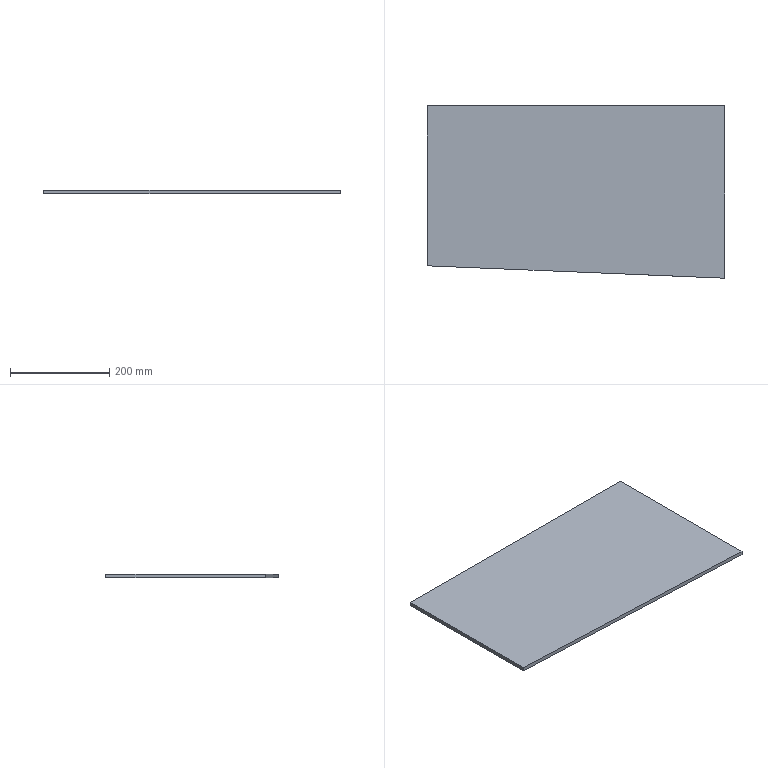Part | STEP file | 04-Middle plate | 1 solid | 6 faces | box 600 x 348 x 8 mm | volume 1609674 mm3 | plane 6
STEP:
#1=CARTESIAN_POINT('',(0.,0.,0.));
#2=DIRECTION('',(0.,0.,1.));
#3=DIRECTION('',(1.,0.,0.));
#4=AXIS2_PLACEMENT_3D('',#1,#2,#3);
#5=CARTESIAN_POINT('',(0.,0.,0.));
#6=VERTEX_POINT('',#5);
#7=CARTESIAN_POINT('',(0.5211,-323.,0.));
#8=VERTEX_POINT('',#7);
#9=CARTESIAN_POINT('',(0.,0.,0.));
#10=DIRECTION('',(0.001613,-1.,0.));
#11=VECTOR('',#10,1.);
#12=LINE('',#9,#11);
#13=CARTESIAN_POINT('',(0.,0.,8.));
#14=DIRECTION('',(1.,0.001613,0.));
#15=DIRECTION('',(-0.001613,1.,0.));
#16=AXIS2_PLACEMENT_3D('',#13,#14,#15);
#17=PLANE('',#16);
#18=CARTESIAN_POINT('',(0.,-8.));
#19=DIRECTION('',(-1.,0.));
#20=VECTOR('',#19,1.);
#21=LINE('',#18,#20);
#22=(GEOMETRIC_REPRESENTATION_CONTEXT(2)PARAMETRIC_REPRESENTATION_CONTEXT()REPRESENTATION_CONTEXT('',''));
#23=DEFINITIONAL_REPRESENTATION('',(#21),#22);
#24=PCURVE('',#17,#23);
#25=CARTESIAN_POINT('',(0.,0.,0.));
#26=DIRECTION('',(0.,0.,1.));
#27=DIRECTION('',(1.,0.,0.));
#28=AXIS2_PLACEMENT_3D('',#25,#26,#27);
#29=PLANE('',#28);
#30=CARTESIAN_POINT('',(0.,0.));
#31=DIRECTION('',(0.001613,-1.));
#32=VECTOR('',#31,1.);
#33=LINE('',#30,#32);
#34=(GEOMETRIC_REPRESENTATION_CONTEXT(2)PARAMETRIC_REPRESENTATION_CONTEXT()REPRESENTATION_CONTEXT('',''));
#35=DEFINITIONAL_REPRESENTATION('',(#33),#34);
#36=PCURVE('',#29,#35);
#37=SURFACE_CURVE('',#12,(#24,#36),.PCURVE_S1.);
#38=EDGE_CURVE('',#6,#8,#37,.T.);
#39=ORIENTED_EDGE('',*,*,#38,.T.);
#40=CARTESIAN_POINT('',(0.5211,-323.,8.));
#41=VERTEX_POINT('',#40);
#42=CARTESIAN_POINT('',(0.5211,-323.,8.));
#43=DIRECTION('',(0.,0.,-1.));
#44=VECTOR('',#43,1.);
#45=LINE('',#42,#44);
#46=CARTESIAN_POINT('',(-323.,0.));
#47=DIRECTION('',(0.,-1.));
#48=VECTOR('',#47,1.);
#49=LINE('',#46,#48);
#50=(GEOMETRIC_REPRESENTATION_CONTEXT(2)PARAMETRIC_REPRESENTATION_CONTEXT()REPRESENTATION_CONTEXT('',''));
#51=DEFINITIONAL_REPRESENTATION('',(#49),#50);
#52=PCURVE('',#17,#51);
#53=CARTESIAN_POINT('',(0.5211,-323.,8.));
#54=DIRECTION('',(0.04167,0.9991,0.));
#55=DIRECTION('',(-0.9991,0.04167,0.));
#56=AXIS2_PLACEMENT_3D('',#53,#54,#55);
#57=PLANE('',#56);
#58=CARTESIAN_POINT('',(0.,0.));
#59=DIRECTION('',(0.,-1.));
#60=VECTOR('',#59,1.);
#61=LINE('',#58,#60);
#62=(GEOMETRIC_REPRESENTATION_CONTEXT(2)PARAMETRIC_REPRESENTATION_CONTEXT()REPRESENTATION_CONTEXT('',''));
#63=DEFINITIONAL_REPRESENTATION('',(#61),#62);
#64=PCURVE('',#57,#63);
#65=SURFACE_CURVE('',#45,(#52,#64),.PCURVE_S1.);
#66=EDGE_CURVE('',#41,#8,#65,.T.);
#67=ORIENTED_EDGE('',*,*,#66,.F.);
#68=CARTESIAN_POINT('',(0.,0.,8.));
#69=VERTEX_POINT('',#68);
#70=CARTESIAN_POINT('',(0.,0.,8.));
#71=DIRECTION('',(0.001613,-1.,0.));
#72=VECTOR('',#71,1.);
#73=LINE('',#70,#72);
#74=CARTESIAN_POINT('',(0.,0.));
#75=DIRECTION('',(-1.,0.));
#76=VECTOR('',#75,1.);
#77=LINE('',#74,#76);
#78=(GEOMETRIC_REPRESENTATION_CONTEXT(2)PARAMETRIC_REPRESENTATION_CONTEXT()REPRESENTATION_CONTEXT('',''));
#79=DEFINITIONAL_REPRESENTATION('',(#77),#78);
#80=PCURVE('',#17,#79);
#81=CARTESIAN_POINT('',(0.,0.,8.));
#82=DIRECTION('',(0.,0.,1.));
#83=DIRECTION('',(1.,0.,0.));
#84=AXIS2_PLACEMENT_3D('',#81,#82,#83);
#85=PLANE('',#84);
#86=CARTESIAN_POINT('',(0.,0.));
#87=DIRECTION('',(0.001613,-1.));
#88=VECTOR('',#87,1.);
#89=LINE('',#86,#88);
#90=(GEOMETRIC_REPRESENTATION_CONTEXT(2)PARAMETRIC_REPRESENTATION_CONTEXT()REPRESENTATION_CONTEXT('',''));
#91=DEFINITIONAL_REPRESENTATION('',(#89),#90);
#92=PCURVE('',#85,#91);
#93=SURFACE_CURVE('',#73,(#80,#92),.PCURVE_S1.);
#94=EDGE_CURVE('',#69,#41,#93,.T.);
#95=ORIENTED_EDGE('',*,*,#94,.F.);
#96=CARTESIAN_POINT('',(0.,0.,8.));
#97=DIRECTION('',(0.,0.,-1.));
#98=VECTOR('',#97,1.);
#99=LINE('',#96,#98);
#100=CARTESIAN_POINT('',(0.,0.));
#101=DIRECTION('',(0.,-1.));
#102=VECTOR('',#101,1.);
#103=LINE('',#100,#102);
#104=(GEOMETRIC_REPRESENTATION_CONTEXT(2)PARAMETRIC_REPRESENTATION_CONTEXT()REPRESENTATION_CONTEXT('',''));
#105=DEFINITIONAL_REPRESENTATION('',(#103),#104);
#106=PCURVE('',#17,#105);
#107=CARTESIAN_POINT('',(0.,0.,8.));
#108=DIRECTION('',(0.,-1.,0.));
#109=DIRECTION('',(0.,0.,-1.));
#110=AXIS2_PLACEMENT_3D('',#107,#108,#109);
#111=PLANE('',#110);
#112=CARTESIAN_POINT('',(0.,0.));
#113=DIRECTION('',(1.,0.));
#114=VECTOR('',#113,1.);
#115=LINE('',#112,#114);
#116=(GEOMETRIC_REPRESENTATION_CONTEXT(2)PARAMETRIC_REPRESENTATION_CONTEXT()REPRESENTATION_CONTEXT('',''));
#117=DEFINITIONAL_REPRESENTATION('',(#115),#116);
#118=PCURVE('',#111,#117);
#119=SURFACE_CURVE('',#99,(#106,#118),.PCURVE_S1.);
#120=EDGE_CURVE('',#69,#6,#119,.T.);
#121=ORIENTED_EDGE('',*,*,#120,.T.);
#122=EDGE_LOOP('',(#39,#67,#95,#121));
#123=FACE_BOUND('',#122,.T.);
#124=ADVANCED_FACE('',(#123),#17,.F.);
#125=CARTESIAN_POINT('',(600.,-348.,0.));
#126=VERTEX_POINT('',#125);
#127=CARTESIAN_POINT('',(0.5211,-323.,0.));
#128=DIRECTION('',(0.9991,-0.04167,0.));
#129=VECTOR('',#128,1.);
#130=LINE('',#127,#129);
#131=CARTESIAN_POINT('',(0.,-8.));
#132=DIRECTION('',(-1.,0.));
#133=VECTOR('',#132,1.);
#134=LINE('',#131,#133);
#135=(GEOMETRIC_REPRESENTATION_CONTEXT(2)PARAMETRIC_REPRESENTATION_CONTEXT()REPRESENTATION_CONTEXT('',''));
#136=DEFINITIONAL_REPRESENTATION('',(#134),#135);
#137=PCURVE('',#57,#136);
#138=CARTESIAN_POINT('',(0.5211,-323.));
#139=DIRECTION('',(0.9991,-0.04167));
#140=VECTOR('',#139,1.);
#141=LINE('',#138,#140);
#142=(GEOMETRIC_REPRESENTATION_CONTEXT(2)PARAMETRIC_REPRESENTATION_CONTEXT()REPRESENTATION_CONTEXT('',''));
#143=DEFINITIONAL_REPRESENTATION('',(#141),#142);
#144=PCURVE('',#29,#143);
#145=SURFACE_CURVE('',#130,(#137,#144),.PCURVE_S1.);
#146=EDGE_CURVE('',#8,#126,#145,.T.);
#147=ORIENTED_EDGE('',*,*,#146,.T.);
#148=CARTESIAN_POINT('',(600.,-348.,8.));
#149=VERTEX_POINT('',#148);
#150=CARTESIAN_POINT('',(600.,-348.,8.));
#151=DIRECTION('',(0.,0.,-1.));
#152=VECTOR('',#151,1.);
#153=LINE('',#150,#152);
#154=CARTESIAN_POINT('',(-600.,0.));
#155=DIRECTION('',(0.,-1.));
#156=VECTOR('',#155,1.);
#157=LINE('',#154,#156);
#158=(GEOMETRIC_REPRESENTATION_CONTEXT(2)PARAMETRIC_REPRESENTATION_CONTEXT()REPRESENTATION_CONTEXT('',''));
#159=DEFINITIONAL_REPRESENTATION('',(#157),#158);
#160=PCURVE('',#57,#159);
#161=CARTESIAN_POINT('',(600.,0.,8.));
#162=DIRECTION('',(-1.,0.,0.));
#163=DIRECTION('',(0.,-1.,0.));
#164=AXIS2_PLACEMENT_3D('',#161,#162,#163);
#165=PLANE('',#164);
#166=CARTESIAN_POINT('',(348.,0.));
#167=DIRECTION('',(0.,-1.));
#168=VECTOR('',#167,1.);
#169=LINE('',#166,#168);
#170=(GEOMETRIC_REPRESENTATION_CONTEXT(2)PARAMETRIC_REPRESENTATION_CONTEXT()REPRESENTATION_CONTEXT('',''));
#171=DEFINITIONAL_REPRESENTATION('',(#169),#170);
#172=PCURVE('',#165,#171);
#173=SURFACE_CURVE('',#153,(#160,#172),.PCURVE_S1.);
#174=EDGE_CURVE('',#149,#126,#173,.T.);
#175=ORIENTED_EDGE('',*,*,#174,.F.);
#176=CARTESIAN_POINT('',(0.5211,-323.,8.));
#177=DIRECTION('',(0.9991,-0.04167,0.));
#178=VECTOR('',#177,1.);
#179=LINE('',#176,#178);
#180=CARTESIAN_POINT('',(0.,0.));
#181=DIRECTION('',(-1.,0.));
#182=VECTOR('',#181,1.);
#183=LINE('',#180,#182);
#184=(GEOMETRIC_REPRESENTATION_CONTEXT(2)PARAMETRIC_REPRESENTATION_CONTEXT()REPRESENTATION_CONTEXT('',''));
#185=DEFINITIONAL_REPRESENTATION('',(#183),#184);
#186=PCURVE('',#57,#185);
#187=CARTESIAN_POINT('',(0.5211,-323.));
#188=DIRECTION('',(0.9991,-0.04167));
#189=VECTOR('',#188,1.);
#190=LINE('',#187,#189);
#191=(GEOMETRIC_REPRESENTATION_CONTEXT(2)PARAMETRIC_REPRESENTATION_CONTEXT()REPRESENTATION_CONTEXT('',''));
#192=DEFINITIONAL_REPRESENTATION('',(#190),#191);
#193=PCURVE('',#85,#192);
#194=SURFACE_CURVE('',#179,(#186,#193),.PCURVE_S1.);
#195=EDGE_CURVE('',#41,#149,#194,.T.);
#196=ORIENTED_EDGE('',*,*,#195,.F.);
#197=ORIENTED_EDGE('',*,*,#66,.T.);
#198=EDGE_LOOP('',(#147,#175,#196,#197));
#199=FACE_BOUND('',#198,.T.);
#200=ADVANCED_FACE('',(#199),#57,.F.);
#201=CARTESIAN_POINT('',(600.,0.,0.));
#202=VERTEX_POINT('',#201);
#203=CARTESIAN_POINT('',(600.,0.,0.));
#204=DIRECTION('',(0.,1.,0.));
#205=VECTOR('',#204,1.);
#206=LINE('',#203,#205);
#207=CARTESIAN_POINT('',(0.,-8.));
#208=DIRECTION('',(-1.,0.));
#209=VECTOR('',#208,1.);
#210=LINE('',#207,#209);
#211=(GEOMETRIC_REPRESENTATION_CONTEXT(2)PARAMETRIC_REPRESENTATION_CONTEXT()REPRESENTATION_CONTEXT('',''));
#212=DEFINITIONAL_REPRESENTATION('',(#210),#211);
#213=PCURVE('',#165,#212);
#214=CARTESIAN_POINT('',(600.,0.));
#215=DIRECTION('',(0.,1.));
#216=VECTOR('',#215,1.);
#217=LINE('',#214,#216);
#218=(GEOMETRIC_REPRESENTATION_CONTEXT(2)PARAMETRIC_REPRESENTATION_CONTEXT()REPRESENTATION_CONTEXT('',''));
#219=DEFINITIONAL_REPRESENTATION('',(#217),#218);
#220=PCURVE('',#29,#219);
#221=SURFACE_CURVE('',#206,(#213,#220),.PCURVE_S1.);
#222=EDGE_CURVE('',#126,#202,#221,.T.);
#223=ORIENTED_EDGE('',*,*,#222,.T.);
#224=CARTESIAN_POINT('',(600.,0.,8.));
#225=VERTEX_POINT('',#224);
#226=CARTESIAN_POINT('',(600.,0.,8.));
#227=DIRECTION('',(0.,0.,-1.));
#228=VECTOR('',#227,1.);
#229=LINE('',#226,#228);
#230=CARTESIAN_POINT('',(0.,0.));
#231=DIRECTION('',(0.,-1.));
#232=VECTOR('',#231,1.);
#233=LINE('',#230,#232);
#234=(GEOMETRIC_REPRESENTATION_CONTEXT(2)PARAMETRIC_REPRESENTATION_CONTEXT()REPRESENTATION_CONTEXT('',''));
#235=DEFINITIONAL_REPRESENTATION('',(#233),#234);
#236=PCURVE('',#165,#235);
#237=CARTESIAN_POINT('',(0.,600.));
#238=DIRECTION('',(1.,0.));
#239=VECTOR('',#238,1.);
#240=LINE('',#237,#239);
#241=(GEOMETRIC_REPRESENTATION_CONTEXT(2)PARAMETRIC_REPRESENTATION_CONTEXT()REPRESENTATION_CONTEXT('',''));
#242=DEFINITIONAL_REPRESENTATION('',(#240),#241);
#243=PCURVE('',#111,#242);
#244=SURFACE_CURVE('',#229,(#236,#243),.PCURVE_S1.);
#245=EDGE_CURVE('',#225,#202,#244,.T.);
#246=ORIENTED_EDGE('',*,*,#245,.F.);
#247=CARTESIAN_POINT('',(600.,0.,8.));
#248=DIRECTION('',(0.,1.,0.));
#249=VECTOR('',#248,1.);
#250=LINE('',#247,#249);
#251=CARTESIAN_POINT('',(0.,0.));
#252=DIRECTION('',(-1.,0.));
#253=VECTOR('',#252,1.);
#254=LINE('',#251,#253);
#255=(GEOMETRIC_REPRESENTATION_CONTEXT(2)PARAMETRIC_REPRESENTATION_CONTEXT()REPRESENTATION_CONTEXT('',''));
#256=DEFINITIONAL_REPRESENTATION('',(#254),#255);
#257=PCURVE('',#165,#256);
#258=CARTESIAN_POINT('',(600.,0.));
#259=DIRECTION('',(0.,1.));
#260=VECTOR('',#259,1.);
#261=LINE('',#258,#260);
#262=(GEOMETRIC_REPRESENTATION_CONTEXT(2)PARAMETRIC_REPRESENTATION_CONTEXT()REPRESENTATION_CONTEXT('',''));
#263=DEFINITIONAL_REPRESENTATION('',(#261),#262);
#264=PCURVE('',#85,#263);
#265=SURFACE_CURVE('',#250,(#257,#264),.PCURVE_S1.);
#266=EDGE_CURVE('',#149,#225,#265,.T.);
#267=ORIENTED_EDGE('',*,*,#266,.F.);
#268=ORIENTED_EDGE('',*,*,#174,.T.);
#269=EDGE_LOOP('',(#223,#246,#267,#268));
#270=FACE_BOUND('',#269,.T.);
#271=ADVANCED_FACE('',(#270),#165,.F.);
#272=CARTESIAN_POINT('',(0.,0.,0.));
#273=DIRECTION('',(-1.,0.,0.));
#274=VECTOR('',#273,1.);
#275=LINE('',#272,#274);
#276=CARTESIAN_POINT('',(8.,0.));
#277=DIRECTION('',(0.,-1.));
#278=VECTOR('',#277,1.);
#279=LINE('',#276,#278);
#280=(GEOMETRIC_REPRESENTATION_CONTEXT(2)PARAMETRIC_REPRESENTATION_CONTEXT()REPRESENTATION_CONTEXT('',''));
#281=DEFINITIONAL_REPRESENTATION('',(#279),#280);
#282=PCURVE('',#111,#281);
#283=CARTESIAN_POINT('',(0.,0.));
#284=DIRECTION('',(-1.,0.));
#285=VECTOR('',#284,1.);
#286=LINE('',#283,#285);
#287=(GEOMETRIC_REPRESENTATION_CONTEXT(2)PARAMETRIC_REPRESENTATION_CONTEXT()REPRESENTATION_CONTEXT('',''));
#288=DEFINITIONAL_REPRESENTATION('',(#286),#287);
#289=PCURVE('',#29,#288);
#290=SURFACE_CURVE('',#275,(#282,#289),.PCURVE_S1.);
#291=EDGE_CURVE('',#202,#6,#290,.T.);
#292=ORIENTED_EDGE('',*,*,#291,.T.);
#293=ORIENTED_EDGE('',*,*,#120,.F.);
#294=CARTESIAN_POINT('',(0.,0.,8.));
#295=DIRECTION('',(-1.,0.,0.));
#296=VECTOR('',#295,1.);
#297=LINE('',#294,#296);
#298=CARTESIAN_POINT('',(0.,0.));
#299=DIRECTION('',(0.,-1.));
#300=VECTOR('',#299,1.);
#301=LINE('',#298,#300);
#302=(GEOMETRIC_REPRESENTATION_CONTEXT(2)PARAMETRIC_REPRESENTATION_CONTEXT()REPRESENTATION_CONTEXT('',''));
#303=DEFINITIONAL_REPRESENTATION('',(#301),#302);
#304=PCURVE('',#111,#303);
#305=CARTESIAN_POINT('',(0.,0.));
#306=DIRECTION('',(-1.,0.));
#307=VECTOR('',#306,1.);
#308=LINE('',#305,#307);
#309=(GEOMETRIC_REPRESENTATION_CONTEXT(2)PARAMETRIC_REPRESENTATION_CONTEXT()REPRESENTATION_CONTEXT('',''));
#310=DEFINITIONAL_REPRESENTATION('',(#308),#309);
#311=PCURVE('',#85,#310);
#312=SURFACE_CURVE('',#297,(#304,#311),.PCURVE_S1.);
#313=EDGE_CURVE('',#225,#69,#312,.T.);
#314=ORIENTED_EDGE('',*,*,#313,.F.);
#315=ORIENTED_EDGE('',*,*,#245,.T.);
#316=EDGE_LOOP('',(#292,#293,#314,#315));
#317=FACE_BOUND('',#316,.T.);
#318=ADVANCED_FACE('',(#317),#111,.F.);
#319=ORIENTED_EDGE('',*,*,#94,.T.);
#320=ORIENTED_EDGE('',*,*,#195,.T.);
#321=ORIENTED_EDGE('',*,*,#266,.T.);
#322=ORIENTED_EDGE('',*,*,#313,.T.);
#323=EDGE_LOOP('',(#319,#320,#321,#322));
#324=FACE_BOUND('',#323,.T.);
#325=ADVANCED_FACE('',(#324),#85,.T.);
#326=ORIENTED_EDGE('',*,*,#38,.F.);
#327=ORIENTED_EDGE('',*,*,#291,.F.);
#328=ORIENTED_EDGE('',*,*,#222,.F.);
#329=ORIENTED_EDGE('',*,*,#146,.F.);
#330=EDGE_LOOP('',(#326,#327,#328,#329));
#331=FACE_BOUND('',#330,.T.);
#332=ADVANCED_FACE('',(#331),#29,.F.);
#333=CLOSED_SHELL('',(#124,#200,#271,#318,#325,#332));
#334=MANIFOLD_SOLID_BREP('',#333);
#335=(LENGTH_UNIT()NAMED_UNIT(*)SI_UNIT(.MILLI.,.METRE.));
#336=UNCERTAINTY_MEASURE_WITH_UNIT(LENGTH_MEASURE(0.0000001),#335,'','');
#337=(NAMED_UNIT(*)PLANE_ANGLE_UNIT()SI_UNIT($,.RADIAN.));
#338=(NAMED_UNIT(*)SI_UNIT($,.STERADIAN.)SOLID_ANGLE_UNIT());
#339=(GEOMETRIC_REPRESENTATION_CONTEXT(3)GLOBAL_UNCERTAINTY_ASSIGNED_CONTEXT((#336))GLOBAL_UNIT_ASSIGNED_CONTEXT((#335,#337,#338))REPRESENTATION_CONTEXT('',''));
#340=ADVANCED_BREP_SHAPE_REPRESENTATION('',(#4,#334),#339);